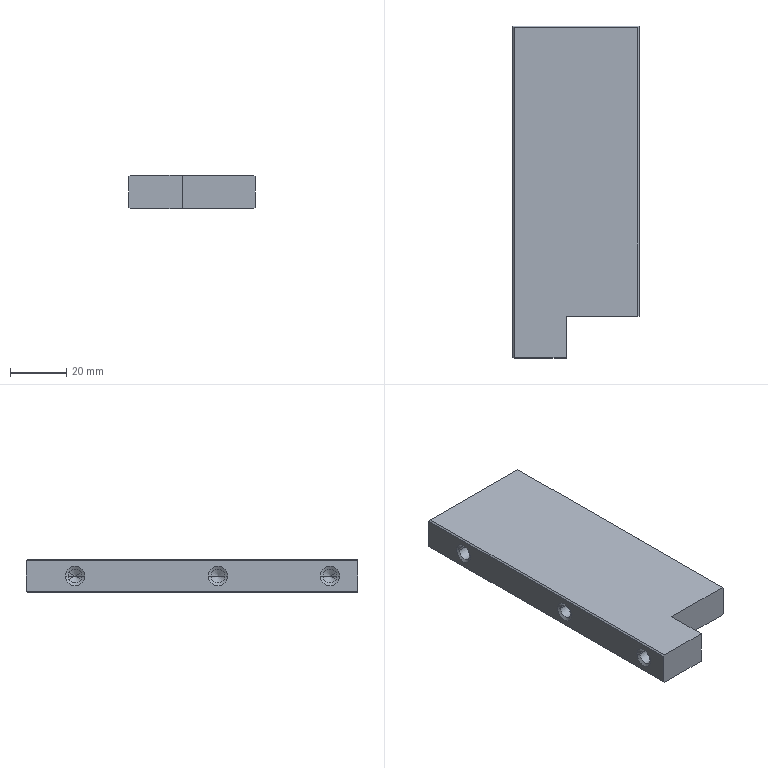Part | NX | 1 solid | 54 faces | box 45 x 118.5 x 12 mm | volume 56934 mm3 | cone 26 | plane 14 | cylinder 14 | commonest cylinder face diameters 5 x14